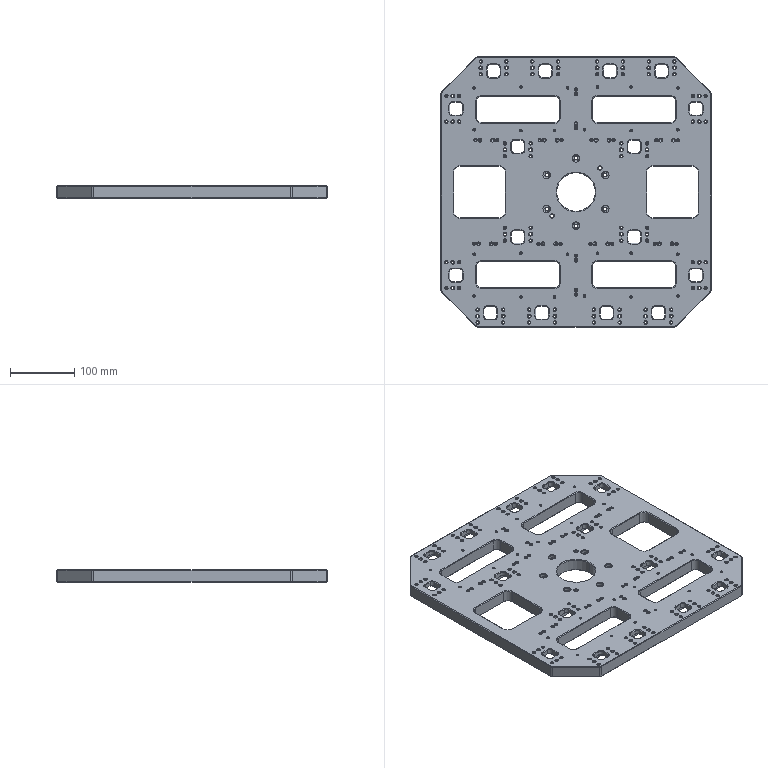Part | SolidWorks | features HoleWzd 5, Chamfer 2, Cut 1, Extrusion 1 | 1 solid | 1562 faces | box 420 x 420 x 20 mm | volume 2237254 mm3 | cone 676 | cylinder 510 | plane 376 | commonest cylinder face diameters 3.3 x168 4 x104 10 x84 14 x64 2.05 x48 16 x16